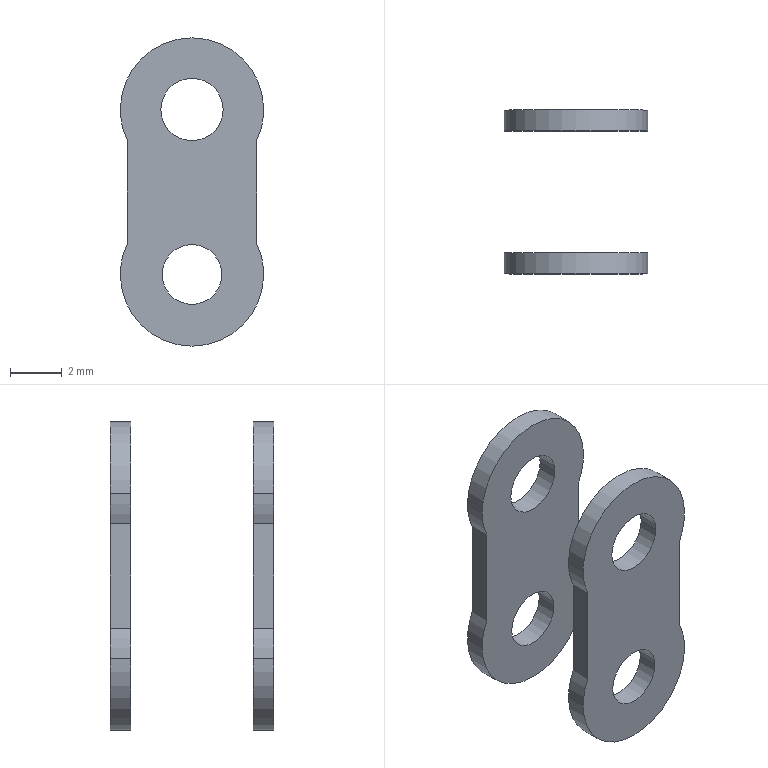Part | SolidWorks | features RefPoint 2 | 2 solids | 28 faces | box 5.52 x 6.3 x 11.87 mm | volume 76.514 mm3 | cylinder 20 | plane 8 | commonest cylinder face diameters 5.52 x12 2.3 x4 2.4 x4